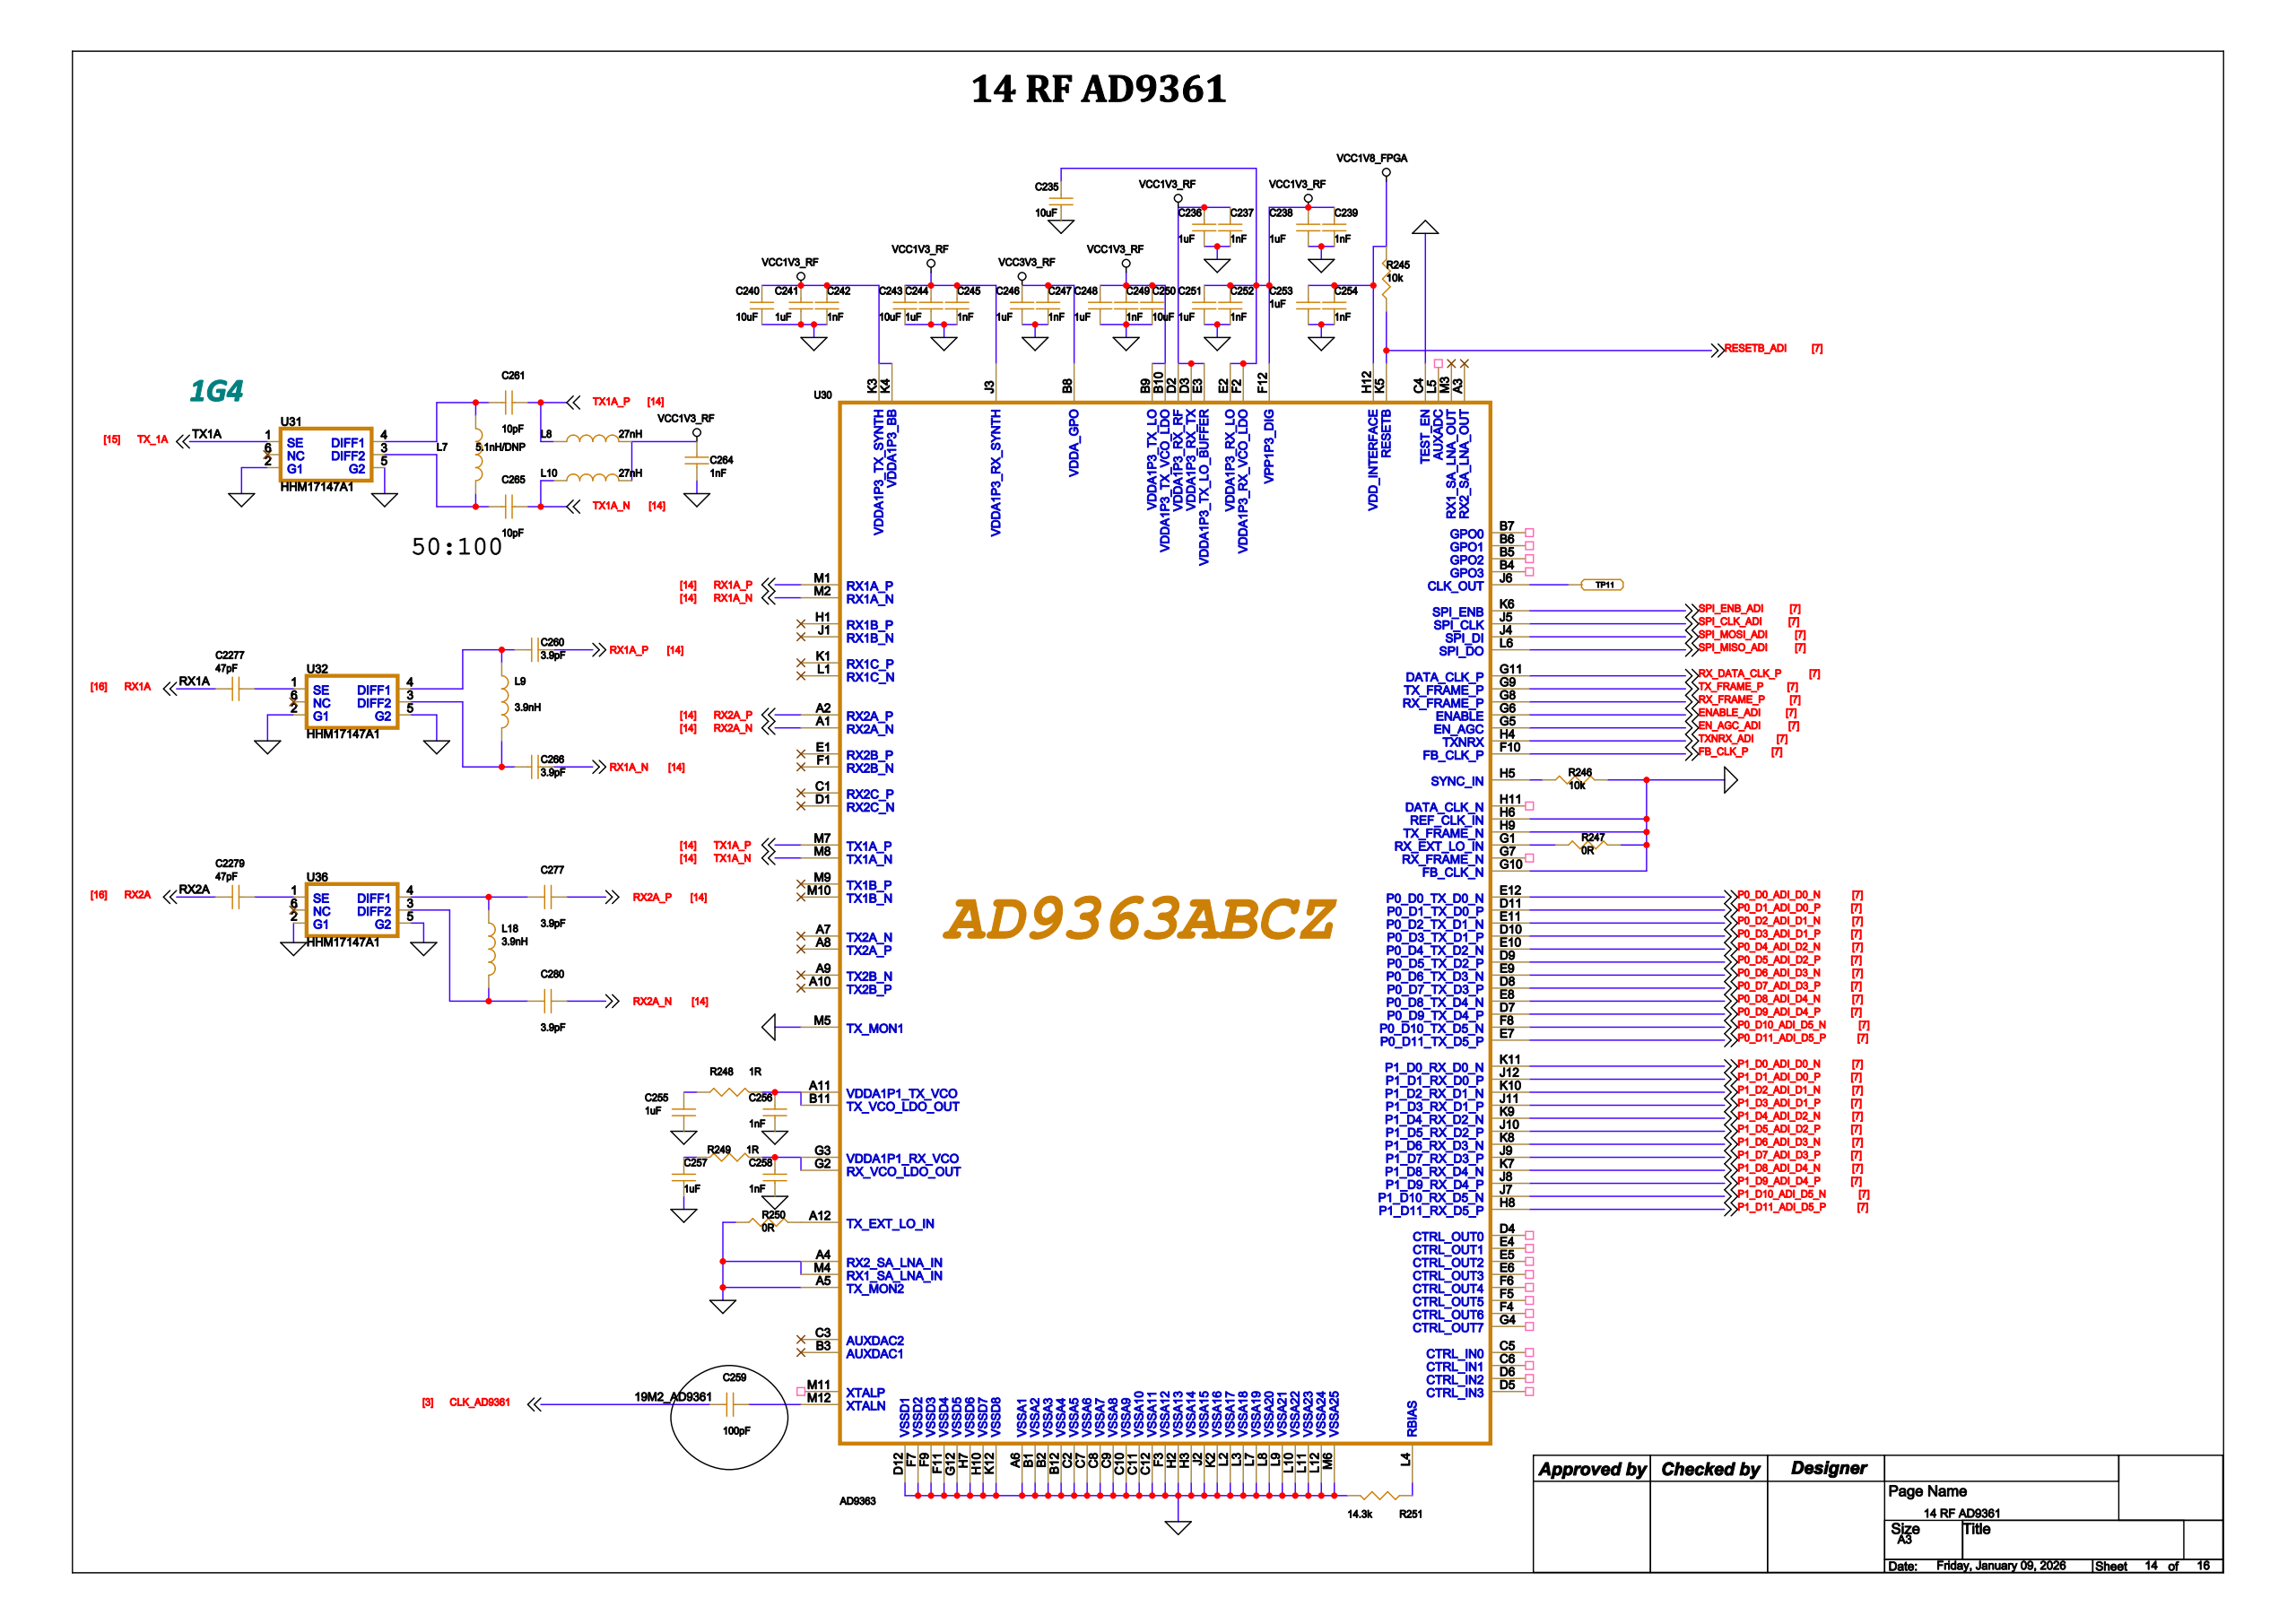Circuit board | Cadence Allegro | 442 parts | 326 nets | one sheet of the schematic
Parts on this sheet (reference | value | footprint):
C235 | 10uF | C0603
C236 | 1uF | C0201
C237 | 1nF | C0201
C238 | 1uF | C0201
C239 | 1nF | C0201
C240 | 10uF | C0603
C241 | 1uF | C0201
C242 | 1nF | C0201
C243 | 10uF | C0603
C244 | 1uF | C0201
C245 | 1nF | C0201
C246 | 1uF | C0201
C247 | 1nF | C0201
C248 | 1uF | C0201
C249 | 1nF | C0201
C250 | 10uF | C0603
C251 | 1uF | C0201
C252 | 1nF | C0201
C253 | 1uF | C0201
C254 | 1nF | C0201
C255 | 1uF | C0201
C256 | 1nF | C0201
C257 | 1uF | C0201
C258 | 1nF | C0201
C259 | 100pF | C0201
C260 | 3.9pF | C0201
C261 | 10pF | C0201
C264 | 1nF | C0201
C265 | 10pF | C0201
C266 | 3.9pF | C0201
C277 | 3.9pF | C0201
C280 | 3.9pF | C0201
C2277 | 47pF | C0201
C2279 | 47pF | C0201
L7 | 5.1nH/DNP | L0201
L8 | 27nH | L0201
L9 | 3.9nH | L0201
L10 | 27nH | L0201
L18 | 3.9nH | L0201
R245 | 10K | R0201
R246 | 10K | R0201
R247 | 0R | R0201
R248 | 1R | R0201
R249 | 1R | R0201
R250 | 0R | R0201
R251 | 14.3k | R0201
TP11 | LABTESTPOINT | LTPT28C49P
U30 | AD9363 | CSPBGA-144-0_8-AD9361
U31 | HHM17147A1 | B1608-LDB18
U32 | HHM17147A1 | B1608-LDB18
U36 | HHM17147A1 | B1608-LDB18
Nets of these parts (net: part-pin ...):
GND: C235-1 C236-1 C237-1 C238-1 C239-1 C240-1 C241-1 C242-1 C243-1 C244-1 C245-1 C246-1 C247-1 C248-1 C249-1 C250-1 C251-1 C252-1 C253-1 C254-1 C255-1 C256-1 C257-1 C258-1 C264-2 R246-2 R247-2 R250-1 R251-2 U31-2 U31-5 U32-2 U32-5 U36-2 U36-5 U30-A4 U30-A5 U30-A6 U30-B1 U30-B2 U30-B12 U30-C2 U30-C4 U30-C7 U30-C8 U30-C9 U30-C10 U30-C11 U30-C12 U30-D12 U30-F3 U30-F7 U30-F9 U30-F11 U30-G10 U30-G12 U30-H2 U30-H3 U30-H6 U30-H7 U30-H9 U30-H10 U30-J2 U30-K2 U30-K12 U30-L2 U30-L3 U30-L7 U30-L8 U30-L9 U30-L10 U30-L11 U30-L12 U30-M4 U30-M5 U30-M6
VCC3V3_RF: C246-2 C247-2 U30-B8
VCC1V8_FPGA: C253-2 C254-2 R245-2 U30-H12
RX1A: C2277-2
RX2A: C2279-2
TX1A_N: C265-1 L10-1 U30-M8
VCC1V3_RF: C235-2 C236-2 C237-2 C238-2 C239-2 C240-2 C241-2 C242-2 C243-2 C244-2 C245-2 C248-2 C249-2 C250-2 C251-2 C252-2 C264-1 L8-2 L10-2 U30-B9 U30-B10 U30-D2 U30-D3 U30-E2 U30-E3 U30-F2 U30-F12 U30-J3 U30-K3 U30-K4
TX1A_P: C261-1 L8-1 U30-M7
N50580135: C277-2 L18-1 U36-4
N50580143: C280-2 L18-2 U36-3
N50579732: C260-2 L9-1 U32-4
N50579777: C266-2 L9-2 U32-3
N50578806: C261-2 L7-1 U31-4
N50578863: C265-2 L7-2 U31-3
CLK_AD9361: C259-2
N42518044: C255-2 R248-1
N42517035: C257-2 R249-2
N42517025: C259-1 U30-M12
N50579773: C2277-1 U32-1
N50580133: C2279-1 U36-1
TX_1A: U31-1
N42518038: C256-2 R248-2 U30-A11 U30-B11
N42517037: C258-2 R249-1 U30-G2 U30-G3
RX1A_P: C260-1 U30-M1
RX1A_N: C266-1 U30-M2
RX2A_P: C277-1 U30-A2
RX2A_N: C280-1 U30-A1
RESETB_ADI: R245-1 U30-K5
N42516994: R246-1 U30-H5
N42517021: R247-1 U30-G1
N4284422211: R250-2 U30-A12
N42517959: R251-1 U30-L4
P0_D10_ADI_D5_N: U30-F8
EN_AGC_ADI: U30-G5
P0_D6_ADI_D3_N: U30-E9
RX_DATA_CLK_P: U30-G11
TX_FRAME_P: U30-G9
P1_D5_ADI_D2_P: U30-J10
P1_D8_ADI_D4_N: U30-K7
P1_D10_ADI_D5_N: U30-J7
ENABLE_ADI: U30-G6
TXNRX_ADI: U30-H4
RX_FRAME_P: U30-G8
SPI_MOSI_ADI: U30-J4
SPI_CLK_ADI: U30-J5
P1_D11_ADI_D5_P: U30-H8
P0_D0_ADI_D0_N: U30-E12
P1_D1_ADI_D0_P: U30-J12
SPI_MISO_ADI: U30-L6
P1_D9_ADI_D4_P: U30-J8
P1_D6_ADI_D3_N: U30-K8
P1_D7_ADI_D3_P: U30-J9
SPI_ENB_ADI: U30-K6
P1_D2_ADI_D1_N: U30-K10
P1_D4_ADI_D2_N: U30-K9
P0_D2_ADI_D1_N: U30-E11
P0_D1_ADI_D0_P: U30-D11
P0_D3_ADI_D1_P: U30-D10
FB_CLK_P: U30-F10
P1_D3_ADI_D1_P: U30-J11
P1_D0_ADI_D0_N: U30-K11
P0_D5_ADI_D2_P: U30-D9
P0_D9_ADI_D4_P: U30-D7
P0_D8_ADI_D4_N: U30-E8
P0_D4_ADI_D2_N: U30-E10
P0_D11_ADI_D5_P: U30-E7
P0_D7_ADI_D3_P: U30-D8
N42543260: TP11-1 U30-J6